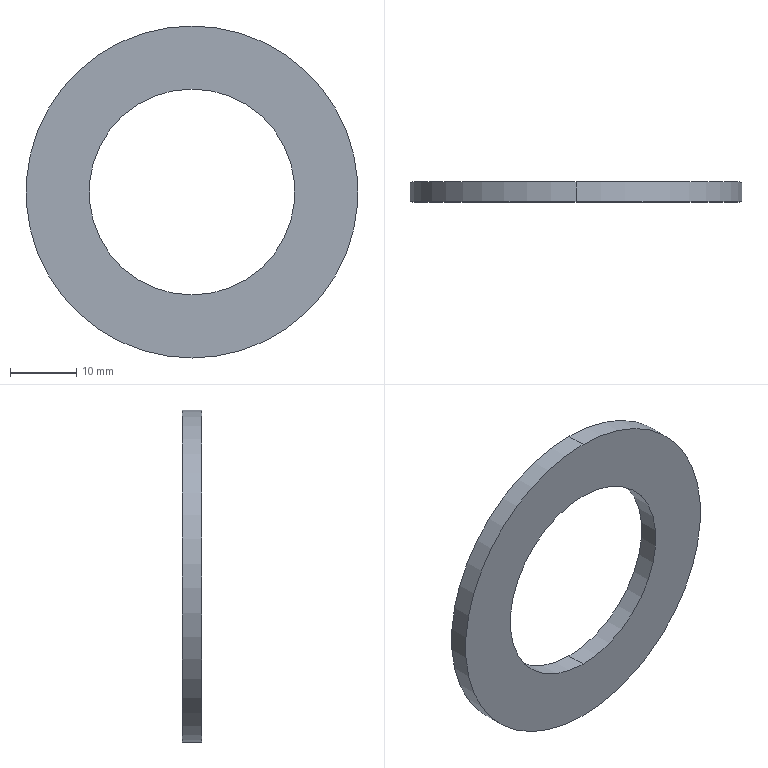Part | SolidWorks | features MirrorStock 1 | 1 solid | 6 faces | box 50 x 3 x 50 mm | volume 3626 mm3 | cylinder 4 | plane 2 | commonest cylinder face diameters 31 x2 50 x2
STEP:
#1=CARTESIAN_POINT('',(0.,1.5,-15.5));
#2=VERTEX_POINT('',#1);
#3=CARTESIAN_POINT('',(0.,1.5,15.5));
#4=VERTEX_POINT('',#3);
#5=CARTESIAN_POINT('',(0.,1.5,0.));
#6=DIRECTION('',(0.,-1.,0.));
#7=DIRECTION('',(0.,0.,-1.));
#8=AXIS2_PLACEMENT_3D('',#5,#6,#7);
#9=CIRCLE('',#8,15.5);
#10=EDGE_CURVE('',#2,#4,#9,.T.);
#11=ORIENTED_EDGE('',*,*,#10,.F.);
#12=CARTESIAN_POINT('',(0.,-1.5,-15.5));
#13=VERTEX_POINT('',#12);
#14=CARTESIAN_POINT('',(0.,1.5,-15.5));
#15=DIRECTION('',(0.,-1.,0.));
#16=VECTOR('',#15,1000.);
#17=LINE('',#14,#16);
#18=EDGE_CURVE('',#2,#13,#17,.T.);
#19=ORIENTED_EDGE('',*,*,#18,.T.);
#20=CARTESIAN_POINT('',(0.,-1.5,15.5));
#21=VERTEX_POINT('',#20);
#22=CARTESIAN_POINT('',(0.,-1.5,0.));
#23=DIRECTION('',(0.,-1.,0.));
#24=DIRECTION('',(0.,0.,-1.));
#25=AXIS2_PLACEMENT_3D('',#22,#23,#24);
#26=CIRCLE('',#25,15.5);
#27=EDGE_CURVE('',#13,#21,#26,.T.);
#28=ORIENTED_EDGE('',*,*,#27,.T.);
#29=CARTESIAN_POINT('',(0.,1.5,15.5));
#30=DIRECTION('',(0.,-1.,0.));
#31=VECTOR('',#30,1000.);
#32=LINE('',#29,#31);
#33=EDGE_CURVE('',#4,#21,#32,.T.);
#34=ORIENTED_EDGE('',*,*,#33,.F.);
#35=EDGE_LOOP('',(#11,#19,#28,#34));
#36=FACE_OUTER_BOUND('',#35,.T.);
#37=CARTESIAN_POINT('',(0.,1.5,0.));
#38=DIRECTION('',(0.,-1.,0.));
#39=DIRECTION('',(0.,0.,1.));
#40=AXIS2_PLACEMENT_3D('',#37,#38,#39);
#41=CYLINDRICAL_SURFACE('',#40,15.5);
#42=ADVANCED_FACE('',(#36),#41,.F.);
#43=CARTESIAN_POINT('',(0.,1.5,25.));
#44=VERTEX_POINT('',#43);
#45=CARTESIAN_POINT('',(0.,1.5,-25.));
#46=VERTEX_POINT('',#45);
#47=CARTESIAN_POINT('',(0.,1.5,0.));
#48=DIRECTION('',(0.,-1.,0.));
#49=DIRECTION('',(0.,0.,-1.));
#50=AXIS2_PLACEMENT_3D('',#47,#48,#49);
#51=CIRCLE('',#50,25.);
#52=EDGE_CURVE('',#44,#46,#51,.T.);
#53=ORIENTED_EDGE('',*,*,#52,.T.);
#54=CARTESIAN_POINT('',(0.,-1.5,-25.));
#55=VERTEX_POINT('',#54);
#56=CARTESIAN_POINT('',(0.,1.5,-25.));
#57=DIRECTION('',(0.,-1.,0.));
#58=VECTOR('',#57,1000.);
#59=LINE('',#56,#58);
#60=EDGE_CURVE('',#46,#55,#59,.T.);
#61=ORIENTED_EDGE('',*,*,#60,.T.);
#62=CARTESIAN_POINT('',(0.,-1.5,25.));
#63=VERTEX_POINT('',#62);
#64=CARTESIAN_POINT('',(0.,-1.5,0.));
#65=DIRECTION('',(0.,-1.,0.));
#66=DIRECTION('',(0.,0.,-1.));
#67=AXIS2_PLACEMENT_3D('',#64,#65,#66);
#68=CIRCLE('',#67,25.);
#69=EDGE_CURVE('',#63,#55,#68,.T.);
#70=ORIENTED_EDGE('',*,*,#69,.F.);
#71=CARTESIAN_POINT('',(0.,1.5,25.));
#72=DIRECTION('',(0.,-1.,0.));
#73=VECTOR('',#72,1000.);
#74=LINE('',#71,#73);
#75=EDGE_CURVE('',#44,#63,#74,.T.);
#76=ORIENTED_EDGE('',*,*,#75,.F.);
#77=EDGE_LOOP('',(#53,#61,#70,#76));
#78=FACE_OUTER_BOUND('',#77,.T.);
#79=CARTESIAN_POINT('',(0.,1.5,0.));
#80=DIRECTION('',(0.,-1.,0.));
#81=DIRECTION('',(0.,0.,1.));
#82=AXIS2_PLACEMENT_3D('',#79,#80,#81);
#83=CYLINDRICAL_SURFACE('',#82,25.);
#84=ADVANCED_FACE('',(#78),#83,.T.);
#85=ORIENTED_EDGE('',*,*,#52,.F.);
#86=CARTESIAN_POINT('',(0.,1.5,0.));
#87=DIRECTION('',(0.,-1.,0.));
#88=DIRECTION('',(0.,0.,-1.));
#89=AXIS2_PLACEMENT_3D('',#86,#87,#88);
#90=CIRCLE('',#89,25.);
#91=EDGE_CURVE('',#46,#44,#90,.T.);
#92=ORIENTED_EDGE('',*,*,#91,.F.);
#93=EDGE_LOOP('',(#85,#92));
#94=FACE_OUTER_BOUND('',#93,.T.);
#95=CARTESIAN_POINT('',(0.,1.5,0.));
#96=DIRECTION('',(0.,-1.,0.));
#97=DIRECTION('',(0.,0.,-1.));
#98=AXIS2_PLACEMENT_3D('',#95,#96,#97);
#99=CIRCLE('',#98,15.5);
#100=EDGE_CURVE('',#4,#2,#99,.T.);
#101=ORIENTED_EDGE('',*,*,#100,.T.);
#102=ORIENTED_EDGE('',*,*,#10,.T.);
#103=EDGE_LOOP('',(#101,#102));
#104=FACE_BOUND('',#103,.T.);
#105=CARTESIAN_POINT('',(0.,1.5,0.));
#106=DIRECTION('',(0.,1.,0.));
#107=DIRECTION('',(0.,0.,-1.));
#108=AXIS2_PLACEMENT_3D('',#105,#106,#107);
#109=PLANE('',#108);
#110=ADVANCED_FACE('',(#94,#104),#109,.T.);
#111=ORIENTED_EDGE('',*,*,#69,.T.);
#112=CARTESIAN_POINT('',(0.,-1.5,0.));
#113=DIRECTION('',(0.,-1.,0.));
#114=DIRECTION('',(0.,0.,-1.));
#115=AXIS2_PLACEMENT_3D('',#112,#113,#114);
#116=CIRCLE('',#115,25.);
#117=EDGE_CURVE('',#55,#63,#116,.T.);
#118=ORIENTED_EDGE('',*,*,#117,.T.);
#119=EDGE_LOOP('',(#111,#118));
#120=FACE_OUTER_BOUND('',#119,.T.);
#121=CARTESIAN_POINT('',(0.,-1.5,0.));
#122=DIRECTION('',(0.,-1.,0.));
#123=DIRECTION('',(0.,0.,-1.));
#124=AXIS2_PLACEMENT_3D('',#121,#122,#123);
#125=CIRCLE('',#124,15.5);
#126=EDGE_CURVE('',#21,#13,#125,.T.);
#127=ORIENTED_EDGE('',*,*,#126,.F.);
#128=ORIENTED_EDGE('',*,*,#27,.F.);
#129=EDGE_LOOP('',(#127,#128));
#130=FACE_BOUND('',#129,.T.);
#131=CARTESIAN_POINT('',(0.,-1.5,0.));
#132=DIRECTION('',(0.,1.,0.));
#133=DIRECTION('',(0.,0.,-1.));
#134=AXIS2_PLACEMENT_3D('',#131,#132,#133);
#135=PLANE('',#134);
#136=ADVANCED_FACE('',(#120,#130),#135,.F.);
#137=ORIENTED_EDGE('',*,*,#60,.F.);
#138=ORIENTED_EDGE('',*,*,#91,.T.);
#139=ORIENTED_EDGE('',*,*,#75,.T.);
#140=ORIENTED_EDGE('',*,*,#117,.F.);
#141=EDGE_LOOP('',(#137,#138,#139,#140));
#142=FACE_OUTER_BOUND('',#141,.T.);
#143=CARTESIAN_POINT('',(0.,1.5,0.));
#144=DIRECTION('',(0.,-1.,0.));
#145=DIRECTION('',(0.,0.,1.));
#146=AXIS2_PLACEMENT_3D('',#143,#144,#145);
#147=CYLINDRICAL_SURFACE('',#146,25.);
#148=ADVANCED_FACE('',(#142),#147,.T.);
#149=ORIENTED_EDGE('',*,*,#18,.F.);
#150=ORIENTED_EDGE('',*,*,#100,.F.);
#151=ORIENTED_EDGE('',*,*,#33,.T.);
#152=ORIENTED_EDGE('',*,*,#126,.T.);
#153=EDGE_LOOP('',(#149,#150,#151,#152));
#154=FACE_OUTER_BOUND('',#153,.T.);
#155=CARTESIAN_POINT('',(0.,1.5,0.));
#156=DIRECTION('',(0.,-1.,0.));
#157=DIRECTION('',(0.,0.,1.));
#158=AXIS2_PLACEMENT_3D('',#155,#156,#157);
#159=CYLINDRICAL_SURFACE('',#158,15.5);
#160=ADVANCED_FACE('',(#154),#159,.F.);
#161=CLOSED_SHELL('',(#42,#84,#110,#136,#148,#160));
#162=MANIFOLD_SOLID_BREP('',#161);
#163=CARTESIAN_POINT('',(0.,0.,0.));
#164=DIRECTION('',(0.,0.,1.));
#165=DIRECTION('',(1.,0.,0.));
#166=AXIS2_PLACEMENT_3D('',#163,#164,#165);
#167=(LENGTH_UNIT()NAMED_UNIT(*)SI_UNIT(.MILLI.,.METRE.));
#168=UNCERTAINTY_MEASURE_WITH_UNIT(LENGTH_MEASURE(0.00001),#167,'','');
#169=(NAMED_UNIT(*)PLANE_ANGLE_UNIT()SI_UNIT($,.RADIAN.));
#170=(NAMED_UNIT(*)SI_UNIT($,.STERADIAN.)SOLID_ANGLE_UNIT());
#171=(GEOMETRIC_REPRESENTATION_CONTEXT(3)GLOBAL_UNCERTAINTY_ASSIGNED_CONTEXT((#168))GLOBAL_UNIT_ASSIGNED_CONTEXT((#167,#169,#170))REPRESENTATION_CONTEXT('',''));
#172=ADVANCED_BREP_SHAPE_REPRESENTATION('',(#162,#166),#171);